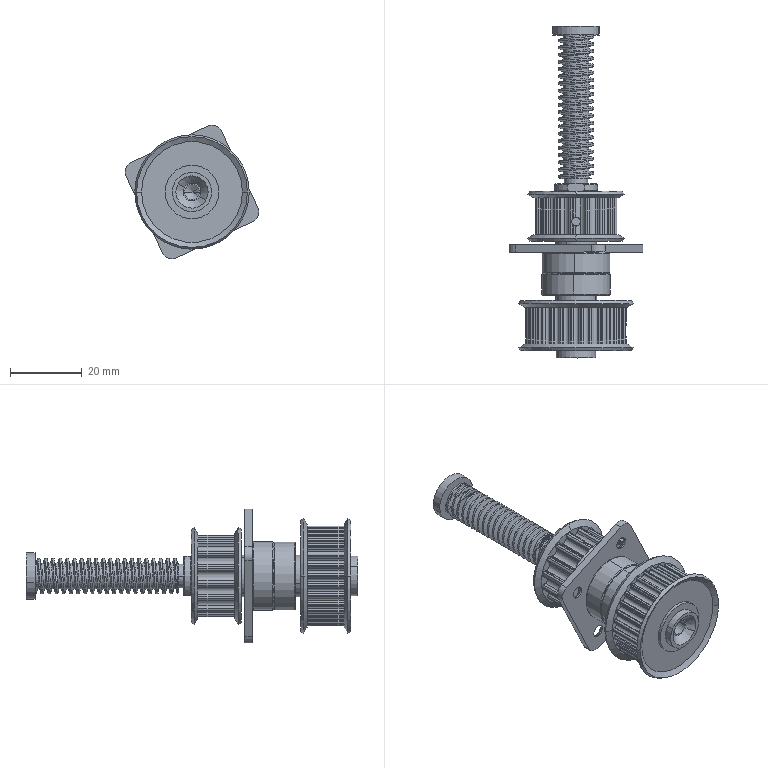Part | NX | features BREP 11 | 14 solids | 805 faces | box 37.314 x 92.5 x 37.314 mm | volume 18812 mm3 | cylinder 477 | sphere 144 | plane 96 | cone 58 | torus 28 | spline 2 | commonest cylinder face diameters 1.02 x118 3.04 x66 1.7 x41 10 x41 27.89 x34 5.08 x33